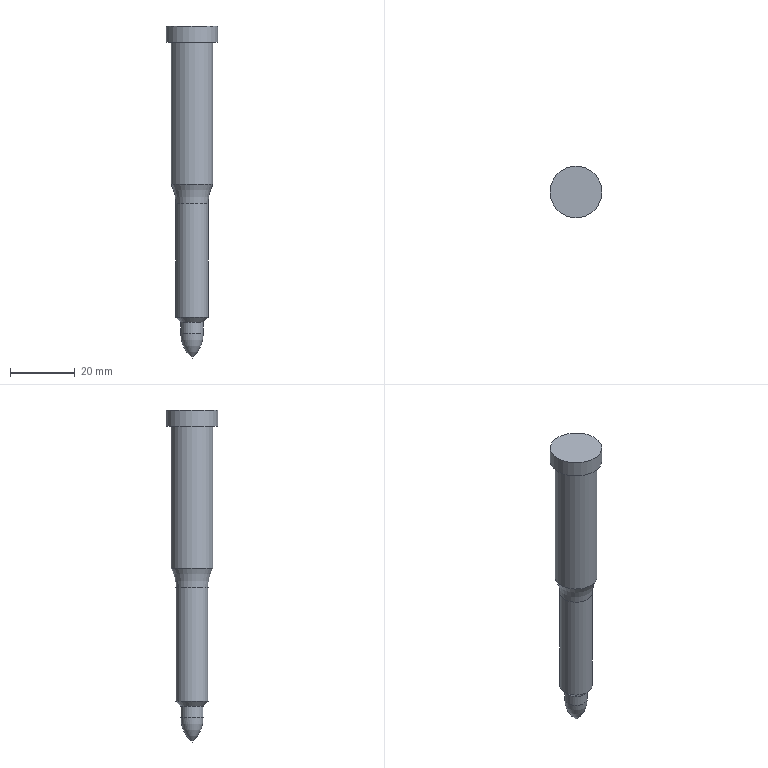Part | NX | features solid 2 | 1 solid | 10 faces | box 16 x 16 x 102.899 mm | volume 10576 mm3 | cylinder 4 | torus 3 | plane 2 | cone 1 | commonest cylinder face diameters 7 x1 10 x1 13 x1 16 x1
STEP:
#1=CARTESIAN_POINT('',(3379.438,-41.938,35.938));
#2=VERTEX_POINT('',#1);
#3=CARTESIAN_POINT('',(3374.438,-41.938,35.938));
#4=DIRECTION('',(0.,0.,-1.));
#5=DIRECTION('',(1.,0.,0.));
#6=AXIS2_PLACEMENT_3D('',#3,#4,#5);
#7=CIRCLE('',#6,5.);
#8=EDGE_CURVE('',#2,#2,#7,.T.);
#9=ORIENTED_EDGE('',*,*,#8,.T.);
#10=EDGE_LOOP('',(#9));
#11=FACE_BOUND('',#10,.T.);
#12=CARTESIAN_POINT('',(3369.438,-41.938,0.7));
#13=VERTEX_POINT('',#12);
#14=CARTESIAN_POINT('',(3374.438,-41.938,0.7));
#15=DIRECTION('',(0.,0.,-1.));
#16=DIRECTION('',(-1.,0.,0.));
#17=AXIS2_PLACEMENT_3D('',#14,#15,#16);
#18=CIRCLE('',#17,5.);
#19=EDGE_CURVE('',#13,#13,#18,.T.);
#20=ORIENTED_EDGE('',*,*,#19,.F.);
#21=EDGE_LOOP('',(#20));
#22=FACE_BOUND('',#21,.T.);
#23=CARTESIAN_POINT('',(3374.438,-41.938,41.));
#24=DIRECTION('',(0.,0.,-1.));
#25=DIRECTION('',(-1.,0.,0.));
#26=AXIS2_PLACEMENT_3D('',#23,#24,#25);
#27=CYLINDRICAL_SURFACE('',#26,5.);
#28=ADVANCED_FACE('',(#11,#22),#27,.T.);
#29=CARTESIAN_POINT('',(3374.438,-41.938,-11.899));
#30=VERTEX_POINT('',#29);
#31=VERTEX_LOOP('',#30);
#32=FACE_BOUND('',#31,.T.);
#33=CARTESIAN_POINT('',(3370.938,-41.938,-4.3));
#34=VERTEX_POINT('',#33);
#35=CARTESIAN_POINT('',(3374.438,-41.938,-4.3));
#36=DIRECTION('',(0.,0.,-1.));
#37=DIRECTION('',(-1.,0.,0.));
#38=AXIS2_PLACEMENT_3D('',#35,#36,#37);
#39=CIRCLE('',#38,3.5);
#40=EDGE_CURVE('',#34,#34,#39,.T.);
#41=ORIENTED_EDGE('',*,*,#40,.T.);
#42=EDGE_LOOP('',(#41));
#43=FACE_BOUND('',#42,.T.);
#44=CARTESIAN_POINT('',(3374.438,-41.938,-4.3));
#45=DIRECTION('',(0.,0.,-1.));
#46=DIRECTION('',(-1.,0.,0.));
#47=AXIS2_PLACEMENT_3D('',#44,#45,#46);
#48=DEGENERATE_TOROIDAL_SURFACE('',#47,6.5,10.,.F.);
#49=ADVANCED_FACE('',(#32,#43),#48,.F.);
#50=CARTESIAN_POINT('',(3370.85,-41.938,-0.7121));
#51=VERTEX_POINT('',#50);
#52=CARTESIAN_POINT('',(3374.438,-41.938,-0.7121));
#53=DIRECTION('',(0.,0.,-1.));
#54=DIRECTION('',(1.,0.,0.));
#55=AXIS2_PLACEMENT_3D('',#52,#53,#54);
#56=CIRCLE('',#55,3.588);
#57=EDGE_CURVE('',#51,#51,#56,.T.);
#58=ORIENTED_EDGE('',*,*,#57,.T.);
#59=EDGE_LOOP('',(#58));
#60=FACE_BOUND('',#59,.T.);
#61=CARTESIAN_POINT('',(3370.938,-41.938,-0.9243));
#62=VERTEX_POINT('',#61);
#63=CARTESIAN_POINT('',(3374.438,-41.938,-0.9243));
#64=DIRECTION('',(0.,0.,1.));
#65=DIRECTION('',(1.,0.,0.));
#66=AXIS2_PLACEMENT_3D('',#63,#64,#65);
#67=CIRCLE('',#66,3.5);
#68=EDGE_CURVE('',#62,#62,#67,.T.);
#69=ORIENTED_EDGE('',*,*,#68,.T.);
#70=EDGE_LOOP('',(#69));
#71=FACE_BOUND('',#70,.T.);
#72=CARTESIAN_POINT('',(3374.438,-41.938,-0.9243));
#73=DIRECTION('',(0.,0.,-1.));
#74=DIRECTION('',(1.,0.,0.));
#75=AXIS2_PLACEMENT_3D('',#72,#73,#74);
#76=TOROIDAL_SURFACE('',#75,3.8,0.3);
#77=ADVANCED_FACE('',(#60,#71),#76,.F.);
#78=ORIENTED_EDGE('',*,*,#40,.F.);
#79=EDGE_LOOP('',(#78));
#80=FACE_BOUND('',#79,.T.);
#81=ORIENTED_EDGE('',*,*,#68,.F.);
#82=EDGE_LOOP('',(#81));
#83=FACE_BOUND('',#82,.T.);
#84=CARTESIAN_POINT('',(3374.438,-41.938,-2.55));
#85=DIRECTION('',(0.,0.,-1.));
#86=DIRECTION('',(-1.,0.,0.));
#87=AXIS2_PLACEMENT_3D('',#84,#85,#86);
#88=CYLINDRICAL_SURFACE('',#87,3.5);
#89=ADVANCED_FACE('',(#80,#83),#88,.T.);
#90=ORIENTED_EDGE('',*,*,#19,.T.);
#91=EDGE_LOOP('',(#90));
#92=FACE_BOUND('',#91,.T.);
#93=ORIENTED_EDGE('',*,*,#57,.F.);
#94=EDGE_LOOP('',(#93));
#95=FACE_BOUND('',#94,.T.);
#96=CARTESIAN_POINT('',(3374.438,-41.938,-0.05));
#97=DIRECTION('',(0.,0.,1.));
#98=DIRECTION('',(-1.,0.,0.));
#99=AXIS2_PLACEMENT_3D('',#96,#97,#98);
#100=CONICAL_SURFACE('',#99,4.25,0.7854);
#101=ADVANCED_FACE('',(#92,#95),#100,.T.);
#102=CARTESIAN_POINT('',(3367.938,-41.938,86.));
#103=VERTEX_POINT('',#102);
#104=CARTESIAN_POINT('',(3374.438,-41.938,86.));
#105=DIRECTION('',(0.,0.,-1.));
#106=DIRECTION('',(-1.,0.,0.));
#107=AXIS2_PLACEMENT_3D('',#104,#105,#106);
#108=CIRCLE('',#107,6.5);
#109=EDGE_CURVE('',#103,#103,#108,.T.);
#110=ORIENTED_EDGE('',*,*,#109,.T.);
#111=EDGE_LOOP('',(#110));
#112=FACE_BOUND('',#111,.T.);
#113=CARTESIAN_POINT('',(3367.938,-41.938,42.));
#114=VERTEX_POINT('',#113);
#115=CARTESIAN_POINT('',(3374.438,-41.938,42.));
#116=DIRECTION('',(0.,0.,-1.));
#117=DIRECTION('',(-1.,0.,0.));
#118=AXIS2_PLACEMENT_3D('',#115,#116,#117);
#119=CIRCLE('',#118,6.5);
#120=EDGE_CURVE('',#114,#114,#119,.T.);
#121=ORIENTED_EDGE('',*,*,#120,.F.);
#122=EDGE_LOOP('',(#121));
#123=FACE_BOUND('',#122,.T.);
#124=CARTESIAN_POINT('',(3374.438,-41.938,86.));
#125=DIRECTION('',(0.,0.,-1.));
#126=DIRECTION('',(1.,0.,0.));
#127=AXIS2_PLACEMENT_3D('',#124,#125,#126);
#128=CYLINDRICAL_SURFACE('',#127,6.5);
#129=ADVANCED_FACE('',(#112,#123),#128,.T.);
#130=CARTESIAN_POINT('',(3382.438,-41.938,91.));
#131=VERTEX_POINT('',#130);
#132=CARTESIAN_POINT('',(3374.438,-41.938,91.));
#133=DIRECTION('',(0.,0.,1.));
#134=DIRECTION('',(1.,0.,0.));
#135=AXIS2_PLACEMENT_3D('',#132,#133,#134);
#136=CIRCLE('',#135,8.);
#137=EDGE_CURVE('',#131,#131,#136,.T.);
#138=ORIENTED_EDGE('',*,*,#137,.T.);
#139=EDGE_LOOP('',(#138));
#140=FACE_BOUND('',#139,.T.);
#141=CARTESIAN_POINT('',(3374.438,-41.938,91.));
#142=DIRECTION('',(0.,0.,1.));
#143=DIRECTION('',(1.,0.,0.));
#144=AXIS2_PLACEMENT_3D('',#141,#142,#143);
#145=PLANE('',#144);
#146=ADVANCED_FACE('',(#140),#145,.T.);
#147=ORIENTED_EDGE('',*,*,#137,.F.);
#148=EDGE_LOOP('',(#147));
#149=FACE_BOUND('',#148,.T.);
#150=CARTESIAN_POINT('',(3366.438,-41.938,86.));
#151=VERTEX_POINT('',#150);
#152=CARTESIAN_POINT('',(3374.438,-41.938,86.));
#153=DIRECTION('',(0.,0.,-1.));
#154=DIRECTION('',(-1.,0.,0.));
#155=AXIS2_PLACEMENT_3D('',#152,#153,#154);
#156=CIRCLE('',#155,8.);
#157=EDGE_CURVE('',#151,#151,#156,.T.);
#158=ORIENTED_EDGE('',*,*,#157,.F.);
#159=EDGE_LOOP('',(#158));
#160=FACE_BOUND('',#159,.T.);
#161=CARTESIAN_POINT('',(3374.438,-41.938,88.5));
#162=DIRECTION('',(0.,0.,-1.));
#163=DIRECTION('',(-1.,0.,0.));
#164=AXIS2_PLACEMENT_3D('',#161,#162,#163);
#165=CYLINDRICAL_SURFACE('',#164,8.);
#166=ADVANCED_FACE('',(#149,#160),#165,.T.);
#167=ORIENTED_EDGE('',*,*,#109,.F.);
#168=EDGE_LOOP('',(#167));
#169=FACE_BOUND('',#168,.T.);
#170=ORIENTED_EDGE('',*,*,#157,.T.);
#171=EDGE_LOOP('',(#170));
#172=FACE_BOUND('',#171,.T.);
#173=CARTESIAN_POINT('',(3374.438,-41.938,86.));
#174=DIRECTION('',(0.,0.,-1.));
#175=DIRECTION('',(-1.,0.,0.));
#176=AXIS2_PLACEMENT_3D('',#173,#174,#175);
#177=PLANE('',#176);
#178=ADVANCED_FACE('',(#169,#172),#177,.T.);
#179=ORIENTED_EDGE('',*,*,#8,.F.);
#180=EDGE_LOOP('',(#179));
#181=FACE_BOUND('',#180,.T.);
#182=ORIENTED_EDGE('',*,*,#120,.T.);
#183=EDGE_LOOP('',(#182));
#184=FACE_BOUND('',#183,.T.);
#185=CARTESIAN_POINT('',(3374.438,-41.938,35.938));
#186=DIRECTION('',(0.,0.,1.));
#187=DIRECTION('',(-1.,0.,0.));
#188=AXIS2_PLACEMENT_3D('',#185,#186,#187);
#189=TOROIDAL_SURFACE('',#188,18.,13.);
#190=ADVANCED_FACE('',(#181,#184),#189,.F.);
#191=CLOSED_SHELL('',(#28,#49,#77,#89,#101,#129,#146,#166,#178,#190));
#192=MANIFOLD_SOLID_BREP('',#191);
#193=(LENGTH_UNIT()NAMED_UNIT(*)SI_UNIT(.MILLI.,.METRE.));
#194=UNCERTAINTY_MEASURE_WITH_UNIT(LENGTH_MEASURE(0.00001),#193,'','');
#195=(NAMED_UNIT(*)PLANE_ANGLE_UNIT()SI_UNIT($,.RADIAN.));
#196=(NAMED_UNIT(*)SI_UNIT($,.STERADIAN.)SOLID_ANGLE_UNIT());
#197=(GEOMETRIC_REPRESENTATION_CONTEXT(3)GLOBAL_UNCERTAINTY_ASSIGNED_CONTEXT((#194))GLOBAL_UNIT_ASSIGNED_CONTEXT((#193,#195,#196))REPRESENTATION_CONTEXT('',''));
#198=ADVANCED_BREP_SHAPE_REPRESENTATION('',(#192),#197);